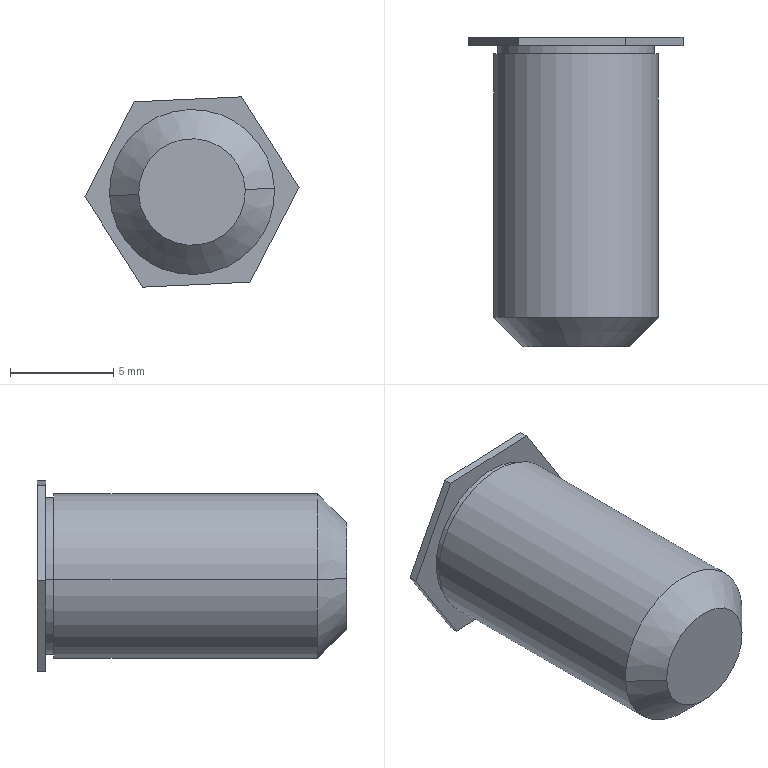Part | NX | features solid 2 | 1 solid | 16 faces | box 10.381 x 15 x 9.23 mm | volume 737.804 mm3 | plane 10 | cylinder 4 | cone 2 | commonest cylinder face diameters 7.6 x2 8 x2
STEP:
#1=CARTESIAN_POINT('',(156.204,-2.9,-887.675));
#2=VERTEX_POINT('',#1);
#3=CARTESIAN_POINT('',(163.796,-2.9,-887.325));
#4=VERTEX_POINT('',#3);
#5=CARTESIAN_POINT('',(160.,-2.9,-887.5));
#6=DIRECTION('',(0.,-1.,0.));
#7=DIRECTION('',(-0.9989,0.,-0.04611));
#8=AXIS2_PLACEMENT_3D('',#5,#6,#7);
#9=CIRCLE('',#8,3.8);
#10=EDGE_CURVE('',#2,#4,#9,.T.);
#11=ORIENTED_EDGE('',*,*,#10,.T.);
#12=CARTESIAN_POINT('',(163.796,-3.3,-887.325));
#13=VERTEX_POINT('',#12);
#14=CARTESIAN_POINT('',(163.796,-2.9,-887.325));
#15=DIRECTION('',(0.,-1.,0.));
#16=VECTOR('',#15,1000.);
#17=LINE('',#14,#16);
#18=EDGE_CURVE('',#4,#13,#17,.T.);
#19=ORIENTED_EDGE('',*,*,#18,.T.);
#20=CARTESIAN_POINT('',(156.204,-3.3,-887.675));
#21=VERTEX_POINT('',#20);
#22=CARTESIAN_POINT('',(160.,-3.3,-887.5));
#23=DIRECTION('',(0.,1.,0.));
#24=DIRECTION('',(0.9989,0.,0.04611));
#25=AXIS2_PLACEMENT_3D('',#22,#23,#24);
#26=CIRCLE('',#25,3.8);
#27=EDGE_CURVE('',#13,#21,#26,.T.);
#28=ORIENTED_EDGE('',*,*,#27,.T.);
#29=CARTESIAN_POINT('',(156.204,-3.3,-887.675));
#30=DIRECTION('',(0.,1.,0.));
#31=VECTOR('',#30,1000.);
#32=LINE('',#29,#31);
#33=EDGE_CURVE('',#21,#2,#32,.T.);
#34=ORIENTED_EDGE('',*,*,#33,.T.);
#35=EDGE_LOOP('',(#11,#19,#28,#34));
#36=FACE_BOUND('',#35,.T.);
#37=CARTESIAN_POINT('',(160.,-3.5,-887.5));
#38=DIRECTION('',(0.,1.,0.));
#39=DIRECTION('',(0.9989,0.,0.04611));
#40=AXIS2_PLACEMENT_3D('',#37,#38,#39);
#41=CYLINDRICAL_SURFACE('',#40,3.8);
#42=ADVANCED_FACE('',(#36),#41,.T.);
#43=CARTESIAN_POINT('',(160.,-3.3,-887.5));
#44=DIRECTION('',(0.,1.,0.));
#45=DIRECTION('',(-0.9989,0.,-0.04611));
#46=AXIS2_PLACEMENT_3D('',#43,#44,#45);
#47=CIRCLE('',#46,3.8);
#48=EDGE_CURVE('',#21,#13,#47,.T.);
#49=ORIENTED_EDGE('',*,*,#48,.T.);
#50=ORIENTED_EDGE('',*,*,#18,.F.);
#51=CARTESIAN_POINT('',(160.,-2.9,-887.5));
#52=DIRECTION('',(0.,-1.,0.));
#53=DIRECTION('',(0.9989,0.,0.04611));
#54=AXIS2_PLACEMENT_3D('',#51,#52,#53);
#55=CIRCLE('',#54,3.8);
#56=EDGE_CURVE('',#4,#2,#55,.T.);
#57=ORIENTED_EDGE('',*,*,#56,.T.);
#58=ORIENTED_EDGE('',*,*,#33,.F.);
#59=EDGE_LOOP('',(#49,#50,#57,#58));
#60=FACE_BOUND('',#59,.T.);
#61=CARTESIAN_POINT('',(160.,-3.5,-887.5));
#62=DIRECTION('',(0.,1.,0.));
#63=DIRECTION('',(0.9989,0.,0.04611));
#64=AXIS2_PLACEMENT_3D('',#61,#62,#63);
#65=CYLINDRICAL_SURFACE('',#64,3.8);
#66=ADVANCED_FACE('',(#60),#65,.T.);
#67=CARTESIAN_POINT('',(154.809,-2.9,-887.74));
#68=VERTEX_POINT('',#67);
#69=CARTESIAN_POINT('',(157.197,-2.9,-883.125));
#70=VERTEX_POINT('',#69);
#71=CARTESIAN_POINT('',(154.809,-2.9,-887.74));
#72=DIRECTION('',(0.4595,0.,0.8882));
#73=VECTOR('',#72,1000.);
#74=LINE('',#71,#73);
#75=EDGE_CURVE('',#68,#70,#74,.T.);
#76=ORIENTED_EDGE('',*,*,#75,.F.);
#77=CARTESIAN_POINT('',(157.612,-2.9,-892.115));
#78=VERTEX_POINT('',#77);
#79=CARTESIAN_POINT('',(157.612,-2.9,-892.115));
#80=DIRECTION('',(-0.5394,0.,0.842));
#81=VECTOR('',#80,1000.);
#82=LINE('',#79,#81);
#83=EDGE_CURVE('',#78,#68,#82,.T.);
#84=ORIENTED_EDGE('',*,*,#83,.F.);
#85=CARTESIAN_POINT('',(162.803,-2.9,-891.875));
#86=VERTEX_POINT('',#85);
#87=CARTESIAN_POINT('',(157.612,-2.9,-892.115));
#88=DIRECTION('',(0.9989,0.,0.04611));
#89=VECTOR('',#88,1000.);
#90=LINE('',#87,#89);
#91=EDGE_CURVE('',#78,#86,#90,.T.);
#92=ORIENTED_EDGE('',*,*,#91,.T.);
#93=CARTESIAN_POINT('',(165.191,-2.9,-887.26));
#94=VERTEX_POINT('',#93);
#95=CARTESIAN_POINT('',(165.191,-2.9,-887.26));
#96=DIRECTION('',(-0.4595,0.,-0.8882));
#97=VECTOR('',#96,1000.);
#98=LINE('',#95,#97);
#99=EDGE_CURVE('',#94,#86,#98,.T.);
#100=ORIENTED_EDGE('',*,*,#99,.F.);
#101=CARTESIAN_POINT('',(162.388,-2.9,-882.885));
#102=VERTEX_POINT('',#101);
#103=CARTESIAN_POINT('',(162.388,-2.9,-882.885));
#104=DIRECTION('',(0.5394,0.,-0.842));
#105=VECTOR('',#104,1000.);
#106=LINE('',#103,#105);
#107=EDGE_CURVE('',#102,#94,#106,.T.);
#108=ORIENTED_EDGE('',*,*,#107,.F.);
#109=CARTESIAN_POINT('',(162.388,-2.9,-882.885));
#110=DIRECTION('',(-0.9989,0.,-0.04611));
#111=VECTOR('',#110,1000.);
#112=LINE('',#109,#111);
#113=EDGE_CURVE('',#102,#70,#112,.T.);
#114=ORIENTED_EDGE('',*,*,#113,.T.);
#115=EDGE_LOOP('',(#76,#84,#92,#100,#108,#114));
#116=FACE_BOUND('',#115,.T.);
#117=ORIENTED_EDGE('',*,*,#56,.F.);
#118=ORIENTED_EDGE('',*,*,#10,.F.);
#119=EDGE_LOOP('',(#117,#118));
#120=FACE_BOUND('',#119,.T.);
#121=CARTESIAN_POINT('',(160.,-2.9,-887.5));
#122=DIRECTION('',(0.,1.,0.));
#123=DIRECTION('',(0.9989,0.,0.04611));
#124=AXIS2_PLACEMENT_3D('',#121,#122,#123);
#125=PLANE('',#124);
#126=ADVANCED_FACE('',(#116,#120),#125,.F.);
#127=CARTESIAN_POINT('',(157.197,-2.5,-883.125));
#128=VERTEX_POINT('',#127);
#129=CARTESIAN_POINT('',(157.197,-2.5,-883.125));
#130=DIRECTION('',(0.,-1.,0.));
#131=VECTOR('',#130,1000.);
#132=LINE('',#129,#131);
#133=EDGE_CURVE('',#128,#70,#132,.T.);
#134=ORIENTED_EDGE('',*,*,#133,.T.);
#135=ORIENTED_EDGE('',*,*,#113,.F.);
#136=CARTESIAN_POINT('',(162.388,-2.5,-882.885));
#137=VERTEX_POINT('',#136);
#138=CARTESIAN_POINT('',(162.388,-2.5,-882.885));
#139=DIRECTION('',(0.,-1.,0.));
#140=VECTOR('',#139,1000.);
#141=LINE('',#138,#140);
#142=EDGE_CURVE('',#137,#102,#141,.T.);
#143=ORIENTED_EDGE('',*,*,#142,.F.);
#144=CARTESIAN_POINT('',(162.388,-2.5,-882.885));
#145=DIRECTION('',(-0.9989,0.,-0.04611));
#146=VECTOR('',#145,1000.);
#147=LINE('',#144,#146);
#148=EDGE_CURVE('',#137,#128,#147,.T.);
#149=ORIENTED_EDGE('',*,*,#148,.T.);
#150=EDGE_LOOP('',(#134,#135,#143,#149));
#151=FACE_BOUND('',#150,.T.);
#152=CARTESIAN_POINT('',(159.792,-2.5,-883.005));
#153=DIRECTION('',(-0.04611,0.,0.9989));
#154=DIRECTION('',(0.9989,0.,0.04611));
#155=AXIS2_PLACEMENT_3D('',#152,#153,#154);
#156=PLANE('',#155);
#157=ADVANCED_FACE('',(#151),#156,.T.);
#158=CARTESIAN_POINT('',(162.803,-2.5,-891.875));
#159=VERTEX_POINT('',#158);
#160=CARTESIAN_POINT('',(165.191,-2.5,-887.26));
#161=VERTEX_POINT('',#160);
#162=CARTESIAN_POINT('',(162.803,-2.5,-891.875));
#163=DIRECTION('',(0.4595,0.,0.8882));
#164=VECTOR('',#163,1000.);
#165=LINE('',#162,#164);
#166=EDGE_CURVE('',#159,#161,#165,.T.);
#167=ORIENTED_EDGE('',*,*,#166,.F.);
#168=CARTESIAN_POINT('',(157.612,-2.5,-892.115));
#169=VERTEX_POINT('',#168);
#170=CARTESIAN_POINT('',(157.612,-2.5,-892.115));
#171=DIRECTION('',(0.9989,0.,0.04611));
#172=VECTOR('',#171,1000.);
#173=LINE('',#170,#172);
#174=EDGE_CURVE('',#169,#159,#173,.T.);
#175=ORIENTED_EDGE('',*,*,#174,.F.);
#176=CARTESIAN_POINT('',(154.809,-2.5,-887.74));
#177=VERTEX_POINT('',#176);
#178=CARTESIAN_POINT('',(154.809,-2.5,-887.74));
#179=DIRECTION('',(0.5394,0.,-0.842));
#180=VECTOR('',#179,1000.);
#181=LINE('',#178,#180);
#182=EDGE_CURVE('',#177,#169,#181,.T.);
#183=ORIENTED_EDGE('',*,*,#182,.F.);
#184=CARTESIAN_POINT('',(157.197,-2.5,-883.125));
#185=DIRECTION('',(-0.4595,0.,-0.8882));
#186=VECTOR('',#185,1000.);
#187=LINE('',#184,#186);
#188=EDGE_CURVE('',#128,#177,#187,.T.);
#189=ORIENTED_EDGE('',*,*,#188,.F.);
#190=ORIENTED_EDGE('',*,*,#148,.F.);
#191=CARTESIAN_POINT('',(165.191,-2.5,-887.26));
#192=DIRECTION('',(-0.5394,0.,0.842));
#193=VECTOR('',#192,1000.);
#194=LINE('',#191,#193);
#195=EDGE_CURVE('',#161,#137,#194,.T.);
#196=ORIENTED_EDGE('',*,*,#195,.F.);
#197=EDGE_LOOP('',(#167,#175,#183,#189,#190,#196));
#198=FACE_BOUND('',#197,.T.);
#199=CARTESIAN_POINT('',(160.,-2.5,-887.5));
#200=DIRECTION('',(0.,-1.,0.));
#201=DIRECTION('',(-0.9989,0.,-0.04611));
#202=AXIS2_PLACEMENT_3D('',#199,#200,#201);
#203=PLANE('',#202);
#204=ADVANCED_FACE('',(#198),#203,.F.);
#205=ORIENTED_EDGE('',*,*,#142,.T.);
#206=ORIENTED_EDGE('',*,*,#107,.T.);
#207=CARTESIAN_POINT('',(165.191,-2.9,-887.26));
#208=DIRECTION('',(0.,1.,0.));
#209=VECTOR('',#208,1000.);
#210=LINE('',#207,#209);
#211=EDGE_CURVE('',#94,#161,#210,.T.);
#212=ORIENTED_EDGE('',*,*,#211,.T.);
#213=ORIENTED_EDGE('',*,*,#195,.T.);
#214=EDGE_LOOP('',(#205,#206,#212,#213));
#215=FACE_BOUND('',#214,.T.);
#216=CARTESIAN_POINT('',(163.789,-2.5,-885.073));
#217=DIRECTION('',(0.842,0.,0.5394));
#218=DIRECTION('',(0.5394,0.,-0.842));
#219=AXIS2_PLACEMENT_3D('',#216,#217,#218);
#220=PLANE('',#219);
#221=ADVANCED_FACE('',(#215),#220,.T.);
#222=ORIENTED_EDGE('',*,*,#211,.F.);
#223=ORIENTED_EDGE('',*,*,#99,.T.);
#224=CARTESIAN_POINT('',(162.803,-2.5,-891.875));
#225=DIRECTION('',(0.,-1.,0.));
#226=VECTOR('',#225,1000.);
#227=LINE('',#224,#226);
#228=EDGE_CURVE('',#159,#86,#227,.T.);
#229=ORIENTED_EDGE('',*,*,#228,.F.);
#230=ORIENTED_EDGE('',*,*,#166,.T.);
#231=EDGE_LOOP('',(#222,#223,#229,#230));
#232=FACE_BOUND('',#231,.T.);
#233=CARTESIAN_POINT('',(163.997,-2.5,-889.568));
#234=DIRECTION('',(0.8882,0.,-0.4595));
#235=DIRECTION('',(-0.4595,0.,-0.8882));
#236=AXIS2_PLACEMENT_3D('',#233,#234,#235);
#237=PLANE('',#236);
#238=ADVANCED_FACE('',(#232),#237,.T.);
#239=ORIENTED_EDGE('',*,*,#228,.T.);
#240=ORIENTED_EDGE('',*,*,#91,.F.);
#241=CARTESIAN_POINT('',(157.612,-2.5,-892.115));
#242=DIRECTION('',(0.,-1.,0.));
#243=VECTOR('',#242,1000.);
#244=LINE('',#241,#243);
#245=EDGE_CURVE('',#169,#78,#244,.T.);
#246=ORIENTED_EDGE('',*,*,#245,.F.);
#247=ORIENTED_EDGE('',*,*,#174,.T.);
#248=EDGE_LOOP('',(#239,#240,#246,#247));
#249=FACE_BOUND('',#248,.T.);
#250=CARTESIAN_POINT('',(160.208,-2.5,-891.995));
#251=DIRECTION('',(0.04611,0.,-0.9989));
#252=DIRECTION('',(-0.9989,0.,-0.04611));
#253=AXIS2_PLACEMENT_3D('',#250,#251,#252);
#254=PLANE('',#253);
#255=ADVANCED_FACE('',(#249),#254,.T.);
#256=ORIENTED_EDGE('',*,*,#245,.T.);
#257=ORIENTED_EDGE('',*,*,#83,.T.);
#258=CARTESIAN_POINT('',(154.809,-2.5,-887.74));
#259=DIRECTION('',(0.,-1.,0.));
#260=VECTOR('',#259,1000.);
#261=LINE('',#258,#260);
#262=EDGE_CURVE('',#177,#68,#261,.T.);
#263=ORIENTED_EDGE('',*,*,#262,.F.);
#264=ORIENTED_EDGE('',*,*,#182,.T.);
#265=EDGE_LOOP('',(#256,#257,#263,#264));
#266=FACE_BOUND('',#265,.T.);
#267=CARTESIAN_POINT('',(156.211,-2.5,-889.927));
#268=DIRECTION('',(-0.842,0.,-0.5394));
#269=DIRECTION('',(-0.5394,0.,0.842));
#270=AXIS2_PLACEMENT_3D('',#267,#268,#269);
#271=PLANE('',#270);
#272=ADVANCED_FACE('',(#266),#271,.T.);
#273=ORIENTED_EDGE('',*,*,#262,.T.);
#274=ORIENTED_EDGE('',*,*,#75,.T.);
#275=ORIENTED_EDGE('',*,*,#133,.F.);
#276=ORIENTED_EDGE('',*,*,#188,.T.);
#277=EDGE_LOOP('',(#273,#274,#275,#276));
#278=FACE_BOUND('',#277,.T.);
#279=CARTESIAN_POINT('',(156.003,-2.5,-885.432));
#280=DIRECTION('',(-0.8882,0.,0.4595));
#281=DIRECTION('',(0.4595,0.,0.8882));
#282=AXIS2_PLACEMENT_3D('',#279,#280,#281);
#283=PLANE('',#282);
#284=ADVANCED_FACE('',(#278),#283,.T.);
#285=CARTESIAN_POINT('',(163.996,-3.3,-887.316));
#286=VERTEX_POINT('',#285);
#287=CARTESIAN_POINT('',(156.004,-3.3,-887.684));
#288=VERTEX_POINT('',#287);
#289=CARTESIAN_POINT('',(160.,-3.3,-887.5));
#290=DIRECTION('',(0.,-1.,0.));
#291=DIRECTION('',(0.9989,0.,0.04611));
#292=AXIS2_PLACEMENT_3D('',#289,#290,#291);
#293=CIRCLE('',#292,4.);
#294=EDGE_CURVE('',#286,#288,#293,.T.);
#295=ORIENTED_EDGE('',*,*,#294,.F.);
#296=CARTESIAN_POINT('',(160.,-3.3,-887.5));
#297=DIRECTION('',(0.,-1.,0.));
#298=DIRECTION('',(-0.9989,0.,-0.04611));
#299=AXIS2_PLACEMENT_3D('',#296,#297,#298);
#300=CIRCLE('',#299,4.);
#301=EDGE_CURVE('',#288,#286,#300,.T.);
#302=ORIENTED_EDGE('',*,*,#301,.F.);
#303=EDGE_LOOP('',(#295,#302));
#304=FACE_BOUND('',#303,.T.);
#305=ORIENTED_EDGE('',*,*,#48,.F.);
#306=ORIENTED_EDGE('',*,*,#27,.F.);
#307=EDGE_LOOP('',(#305,#306));
#308=FACE_BOUND('',#307,.T.);
#309=CARTESIAN_POINT('',(163.996,-3.3,-887.316));
#310=DIRECTION('',(0.,1.,0.));
#311=DIRECTION('',(0.9989,0.,0.04611));
#312=AXIS2_PLACEMENT_3D('',#309,#310,#311);
#313=PLANE('',#312);
#314=ADVANCED_FACE('',(#304,#308),#313,.T.);
#315=ORIENTED_EDGE('',*,*,#301,.T.);
#316=CARTESIAN_POINT('',(163.996,-16.086,-887.316));
#317=VERTEX_POINT('',#316);
#318=CARTESIAN_POINT('',(163.996,-3.3,-887.316));
#319=DIRECTION('',(0.,-1.,0.));
#320=VECTOR('',#319,1000.);
#321=LINE('',#318,#320);
#322=EDGE_CURVE('',#286,#317,#321,.T.);
#323=ORIENTED_EDGE('',*,*,#322,.T.);
#324=CARTESIAN_POINT('',(156.004,-16.086,-887.684));
#325=VERTEX_POINT('',#324);
#326=CARTESIAN_POINT('',(160.,-16.086,-887.5));
#327=DIRECTION('',(0.,1.,0.));
#328=DIRECTION('',(0.9989,0.,0.04611));
#329=AXIS2_PLACEMENT_3D('',#326,#327,#328);
#330=CIRCLE('',#329,4.);
#331=EDGE_CURVE('',#317,#325,#330,.T.);
#332=ORIENTED_EDGE('',*,*,#331,.T.);
#333=CARTESIAN_POINT('',(156.004,-16.086,-887.684));
#334=DIRECTION('',(0.,1.,0.));
#335=VECTOR('',#334,1000.);
#336=LINE('',#333,#335);
#337=EDGE_CURVE('',#325,#288,#336,.T.);
#338=ORIENTED_EDGE('',*,*,#337,.T.);
#339=EDGE_LOOP('',(#315,#323,#332,#338));
#340=FACE_BOUND('',#339,.T.);
#341=CARTESIAN_POINT('',(160.,-3.5,-887.5));
#342=DIRECTION('',(0.,1.,0.));
#343=DIRECTION('',(0.9989,0.,0.04611));
#344=AXIS2_PLACEMENT_3D('',#341,#342,#343);
#345=CYLINDRICAL_SURFACE('',#344,4.);
#346=ADVANCED_FACE('',(#340),#345,.T.);
#347=CARTESIAN_POINT('',(160.,-16.086,-887.5));
#348=DIRECTION('',(0.,1.,0.));
#349=DIRECTION('',(-0.9989,0.,-0.04611));
#350=AXIS2_PLACEMENT_3D('',#347,#348,#349);
#351=CIRCLE('',#350,4.);
#352=EDGE_CURVE('',#325,#317,#351,.T.);
#353=ORIENTED_EDGE('',*,*,#352,.T.);
#354=ORIENTED_EDGE('',*,*,#322,.F.);
#355=ORIENTED_EDGE('',*,*,#294,.T.);
#356=ORIENTED_EDGE('',*,*,#337,.F.);
#357=EDGE_LOOP('',(#353,#354,#355,#356));
#358=FACE_BOUND('',#357,.T.);
#359=CARTESIAN_POINT('',(160.,-3.5,-887.5));
#360=DIRECTION('',(0.,1.,0.));
#361=DIRECTION('',(0.9989,0.,0.04611));
#362=AXIS2_PLACEMENT_3D('',#359,#360,#361);
#363=CYLINDRICAL_SURFACE('',#362,4.);
#364=ADVANCED_FACE('',(#358),#363,.T.);
#365=CARTESIAN_POINT('',(157.417,-17.5,-887.619));
#366=VERTEX_POINT('',#365);
#367=CARTESIAN_POINT('',(162.583,-17.5,-887.381));
#368=VERTEX_POINT('',#367);
#369=CARTESIAN_POINT('',(160.,-17.5,-887.5));
#370=DIRECTION('',(0.,1.,0.));
#371=DIRECTION('',(-0.9989,0.,-0.04611));
#372=AXIS2_PLACEMENT_3D('',#369,#370,#371);
#373=CIRCLE('',#372,2.586);
#374=EDGE_CURVE('',#366,#368,#373,.T.);
#375=ORIENTED_EDGE('',*,*,#374,.T.);
#376=CARTESIAN_POINT('',(163.996,-16.086,-887.316));
#377=DIRECTION('',(-0.7064,-0.7071,-0.03261));
#378=VECTOR('',#377,1000.);
#379=LINE('',#376,#378);
#380=EDGE_CURVE('',#317,#368,#379,.T.);
#381=ORIENTED_EDGE('',*,*,#380,.F.);
#382=ORIENTED_EDGE('',*,*,#352,.F.);
#383=CARTESIAN_POINT('',(157.417,-17.5,-887.619));
#384=DIRECTION('',(-0.7064,0.7071,-0.03261));
#385=VECTOR('',#384,1000.);
#386=LINE('',#383,#385);
#387=EDGE_CURVE('',#366,#325,#386,.T.);
#388=ORIENTED_EDGE('',*,*,#387,.F.);
#389=EDGE_LOOP('',(#375,#381,#382,#388));
#390=FACE_BOUND('',#389,.T.);
#391=CARTESIAN_POINT('',(160.,-16.793,-887.5));
#392=DIRECTION('',(0.,1.,0.));
#393=DIRECTION('',(0.9989,0.,0.04611));
#394=AXIS2_PLACEMENT_3D('',#391,#392,#393);
#395=CONICAL_SURFACE('',#394,3.293,0.7854);
#396=ADVANCED_FACE('',(#390),#395,.T.);
#397=ORIENTED_EDGE('',*,*,#331,.F.);
#398=ORIENTED_EDGE('',*,*,#380,.T.);
#399=CARTESIAN_POINT('',(160.,-17.5,-887.5));
#400=DIRECTION('',(0.,1.,0.));
#401=DIRECTION('',(0.9989,0.,0.04611));
#402=AXIS2_PLACEMENT_3D('',#399,#400,#401);
#403=CIRCLE('',#402,2.586);
#404=EDGE_CURVE('',#368,#366,#403,.T.);
#405=ORIENTED_EDGE('',*,*,#404,.T.);
#406=ORIENTED_EDGE('',*,*,#387,.T.);
#407=EDGE_LOOP('',(#397,#398,#405,#406));
#408=FACE_BOUND('',#407,.T.);
#409=CARTESIAN_POINT('',(160.,-16.793,-887.5));
#410=DIRECTION('',(0.,1.,0.));
#411=DIRECTION('',(0.9989,0.,0.04611));
#412=AXIS2_PLACEMENT_3D('',#409,#410,#411);
#413=CONICAL_SURFACE('',#412,3.293,0.7854);
#414=ADVANCED_FACE('',(#408),#413,.T.);
#415=ORIENTED_EDGE('',*,*,#404,.F.);
#416=ORIENTED_EDGE('',*,*,#374,.F.);
#417=EDGE_LOOP('',(#415,#416));
#418=FACE_BOUND('',#417,.T.);
#419=CARTESIAN_POINT('',(160.,-17.5,-887.5));
#420=DIRECTION('',(0.,-1.,0.));
#421=DIRECTION('',(-0.9989,0.,-0.04611));
#422=AXIS2_PLACEMENT_3D('',#419,#420,#421);
#423=PLANE('',#422);
#424=ADVANCED_FACE('',(#418),#423,.T.);
#425=CLOSED_SHELL('',(#42,#66,#126,#157,#204,#221,#238,#255,#272,#284,#314,#346,#364,#396,#414,#424));
#426=MANIFOLD_SOLID_BREP('',#425);
#427=(LENGTH_UNIT()NAMED_UNIT(*)SI_UNIT(.MILLI.,.METRE.));
#428=UNCERTAINTY_MEASURE_WITH_UNIT(LENGTH_MEASURE(0.00001),#427,'','');
#429=(NAMED_UNIT(*)PLANE_ANGLE_UNIT()SI_UNIT($,.RADIAN.));
#430=(NAMED_UNIT(*)SI_UNIT($,.STERADIAN.)SOLID_ANGLE_UNIT());
#431=(GEOMETRIC_REPRESENTATION_CONTEXT(3)GLOBAL_UNCERTAINTY_ASSIGNED_CONTEXT((#428))GLOBAL_UNIT_ASSIGNED_CONTEXT((#427,#429,#430))REPRESENTATION_CONTEXT('',''));
#432=ADVANCED_BREP_SHAPE_REPRESENTATION('',(#426),#431);